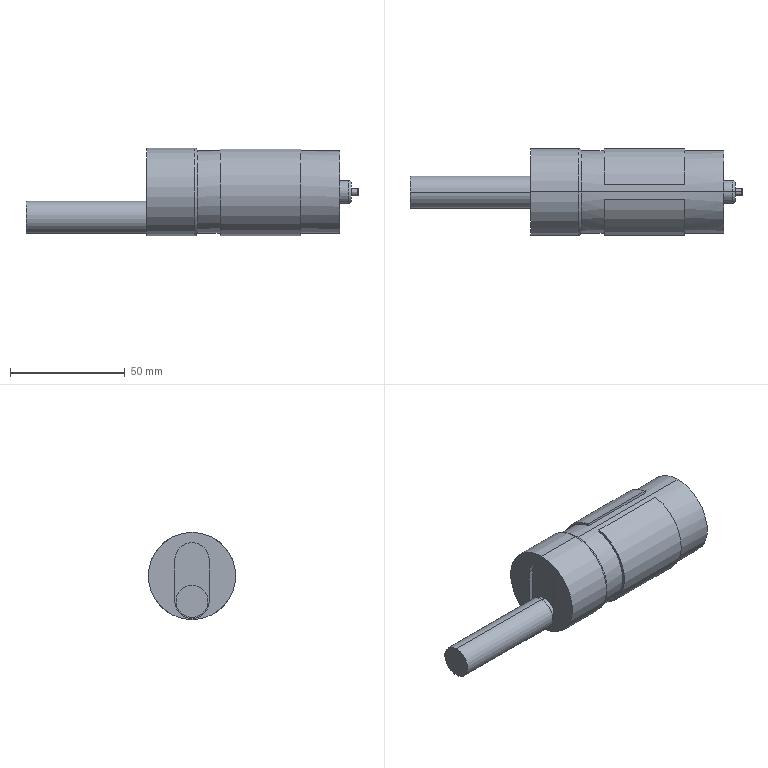Part | SolidWorks | features ICE 13, Fillet 4, Cut 2, Split 2, Chamfer 1, CreateAssemFeat 1, Extrusion 1, MirrorPattern 1, Revolution 1 | 1 solid | 58 faces | box 144.5 x 38 x 38 mm | volume 99346 mm3 | cylinder 27 | plane 25 | torus 6 | commonest cylinder face diameters 12 x5 20.108 x5 38 x4 15 x3 3 x2 10 x2